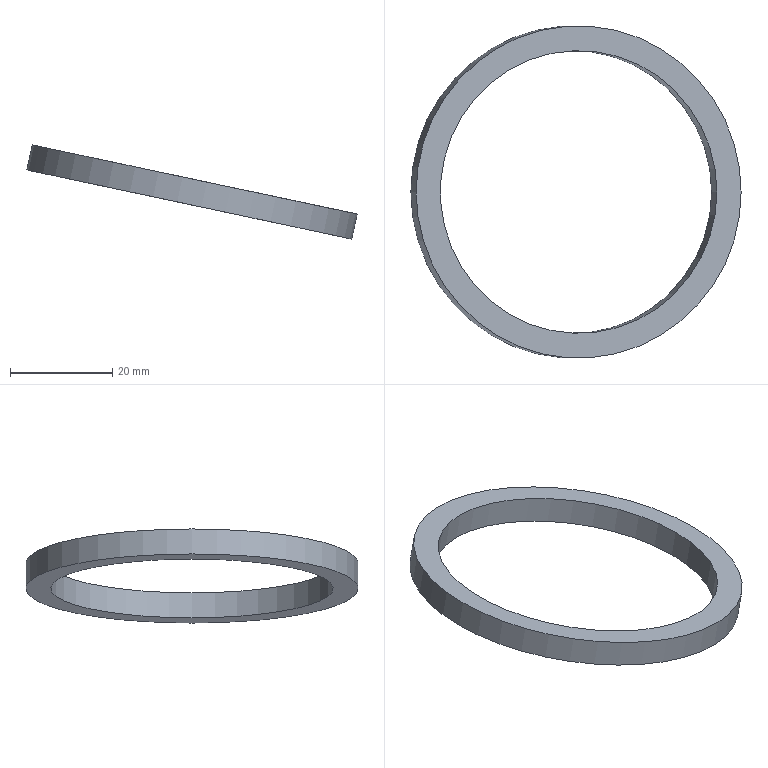Part | STEP file | HL4GZ-1.862.554 (cutter mechanism bushing) | 1 solid | 4 faces | box 64.619 x 65 x 18.405 mm | volume 4582 mm3 | plane 2 | cylinder 2 | commonest cylinder face diameters 55.3 x1 65 x1
STEP:
#1=CARTESIAN_POINT('',(0.,0.,0.));
#2=DIRECTION('',(0.,0.,1.));
#3=DIRECTION('',(1.,0.,0.));
#4=AXIS2_PLACEMENT_3D('',#1,#2,#3);
#5=CARTESIAN_POINT('',(1999.118,0.00003081,-382.69));
#6=VERTEX_POINT('',#5);
#7=CARTESIAN_POINT('',(1972.072,0.00003081,-376.941));
#8=DIRECTION('',(-0.2079,0.,-0.9781));
#9=DIRECTION('',(0.9781,0.,-0.2079));
#10=AXIS2_PLACEMENT_3D('',#7,#8,#9);
#11=CIRCLE('',#10,27.65);
#12=CARTESIAN_POINT('',(1972.072,0.00003081,-376.941));
#13=DIRECTION('',(0.2079,0.,0.9781));
#14=DIRECTION('',(0.,-1.,0.));
#15=AXIS2_PLACEMENT_3D('',#12,#13,#14);
#16=PLANE('',#15);
#17=CARTESIAN_POINT('',(0.,27.65));
#18=CARTESIAN_POINT('',(47.891,27.65));
#19=CARTESIAN_POINT('',(23.946,-13.825));
#20=CARTESIAN_POINT('',(0.,-55.3));
#21=CARTESIAN_POINT('',(-23.946,-13.825));
#22=CARTESIAN_POINT('',(-47.891,27.65));
#23=CARTESIAN_POINT('',(0.,27.65));
#24=(BOUNDED_CURVE()B_SPLINE_CURVE(2,(#17,#18,#19,#20,#21,#22,#23),.UNSPECIFIED.,.T.,.F.)B_SPLINE_CURVE_WITH_KNOTS((1,2,2,2,2,1),(-2.094,0.,2.094,4.189,6.283,8.378),.UNSPECIFIED.)CURVE()GEOMETRIC_REPRESENTATION_ITEM()RATIONAL_B_SPLINE_CURVE((1.,0.5,1.,0.5,1.,0.5,1.))REPRESENTATION_ITEM(''));
#25=(GEOMETRIC_REPRESENTATION_CONTEXT(2)PARAMETRIC_REPRESENTATION_CONTEXT()REPRESENTATION_CONTEXT('',''));
#26=DEFINITIONAL_REPRESENTATION('',(#24),#25);
#27=PCURVE('',#16,#26);
#28=CARTESIAN_POINT('',(1971.033,0.00003081,-381.832));
#29=DIRECTION('',(0.2079,0.,0.9781));
#30=DIRECTION('',(0.,1.,0.));
#31=AXIS2_PLACEMENT_3D('',#28,#29,#30);
#32=CYLINDRICAL_SURFACE('',#31,27.65);
#33=CARTESIAN_POINT('',(10.996,5.));
#34=DIRECTION('',(-1.,0.));
#35=VECTOR('',#34,1.);
#36=LINE('',#33,#35);
#37=(GEOMETRIC_REPRESENTATION_CONTEXT(2)PARAMETRIC_REPRESENTATION_CONTEXT()REPRESENTATION_CONTEXT('',''));
#38=DEFINITIONAL_REPRESENTATION('',(#36),#37);
#39=PCURVE('',#32,#38);
#40=SURFACE_CURVE('',#11,(#27,#39),.PCURVE_S1.);
#41=EDGE_CURVE('',#6,#6,#40,.T.);
#42=ORIENTED_EDGE('',*,*,#41,.T.);
#43=EDGE_LOOP('',(#42));
#44=FACE_BOUND('',#43,.T.);
#45=CARTESIAN_POINT('',(2003.862,0.00003081,-383.698));
#46=VERTEX_POINT('',#45);
#47=CARTESIAN_POINT('',(1972.072,0.00003081,-376.941));
#48=DIRECTION('',(0.2079,0.,0.9781));
#49=DIRECTION('',(0.9781,0.,-0.2079));
#50=AXIS2_PLACEMENT_3D('',#47,#48,#49);
#51=CIRCLE('',#50,32.5);
#52=CARTESIAN_POINT('',(0.,0.));
#53=DIRECTION('',(0.,1.));
#54=AXIS2_PLACEMENT_2D('',#52,#53);
#55=CIRCLE('',#54,32.5);
#56=(GEOMETRIC_REPRESENTATION_CONTEXT(2)PARAMETRIC_REPRESENTATION_CONTEXT()REPRESENTATION_CONTEXT('',''));
#57=DEFINITIONAL_REPRESENTATION('',(#55),#56);
#58=PCURVE('',#16,#57);
#59=CARTESIAN_POINT('',(1971.033,0.00003081,-381.832));
#60=DIRECTION('',(0.2079,0.,0.9781));
#61=DIRECTION('',(0.,1.,0.));
#62=AXIS2_PLACEMENT_3D('',#59,#60,#61);
#63=CYLINDRICAL_SURFACE('',#62,32.5);
#64=CARTESIAN_POINT('',(4.712,5.));
#65=DIRECTION('',(1.,0.));
#66=VECTOR('',#65,1.);
#67=LINE('',#64,#66);
#68=(GEOMETRIC_REPRESENTATION_CONTEXT(2)PARAMETRIC_REPRESENTATION_CONTEXT()REPRESENTATION_CONTEXT('',''));
#69=DEFINITIONAL_REPRESENTATION('',(#67),#68);
#70=PCURVE('',#63,#69);
#71=SURFACE_CURVE('',#51,(#58,#70),.PCURVE_S1.);
#72=EDGE_CURVE('',#46,#46,#71,.T.);
#73=ORIENTED_EDGE('',*,*,#72,.T.);
#74=EDGE_LOOP('',(#73));
#75=FACE_BOUND('',#74,.T.);
#76=ADVANCED_FACE('',(#44,#75),#16,.T.);
#77=CARTESIAN_POINT('',(1998.079,0.00003081,-387.58));
#78=VERTEX_POINT('',#77);
#79=CARTESIAN_POINT('',(1971.033,0.00003081,-381.832));
#80=DIRECTION('',(0.2079,0.,0.9781));
#81=DIRECTION('',(0.9781,0.,-0.2079));
#82=AXIS2_PLACEMENT_3D('',#79,#80,#81);
#83=CIRCLE('',#82,27.65);
#84=CARTESIAN_POINT('',(1971.033,0.00003081,-381.832));
#85=DIRECTION('',(0.2079,0.,0.9781));
#86=DIRECTION('',(0.,-1.,0.));
#87=AXIS2_PLACEMENT_3D('',#84,#85,#86);
#88=PLANE('',#87);
#89=CARTESIAN_POINT('',(0.,0.));
#90=DIRECTION('',(0.,1.));
#91=AXIS2_PLACEMENT_2D('',#89,#90);
#92=CIRCLE('',#91,27.65);
#93=(GEOMETRIC_REPRESENTATION_CONTEXT(2)PARAMETRIC_REPRESENTATION_CONTEXT()REPRESENTATION_CONTEXT('',''));
#94=DEFINITIONAL_REPRESENTATION('',(#92),#93);
#95=PCURVE('',#88,#94);
#96=CARTESIAN_POINT('',(4.712,0.));
#97=DIRECTION('',(1.,0.));
#98=VECTOR('',#97,1.);
#99=LINE('',#96,#98);
#100=(GEOMETRIC_REPRESENTATION_CONTEXT(2)PARAMETRIC_REPRESENTATION_CONTEXT()REPRESENTATION_CONTEXT('',''));
#101=DEFINITIONAL_REPRESENTATION('',(#99),#100);
#102=PCURVE('',#32,#101);
#103=SURFACE_CURVE('',#83,(#95,#102),.PCURVE_S1.);
#104=EDGE_CURVE('',#78,#78,#103,.T.);
#105=ORIENTED_EDGE('',*,*,#104,.T.);
#106=EDGE_LOOP('',(#105));
#107=FACE_BOUND('',#106,.T.);
#108=CARTESIAN_POINT('',(2002.823,0.00003081,-388.589));
#109=VERTEX_POINT('',#108);
#110=CARTESIAN_POINT('',(1971.033,0.00003081,-381.832));
#111=DIRECTION('',(-0.2079,0.,-0.9781));
#112=DIRECTION('',(0.9781,0.,-0.2079));
#113=AXIS2_PLACEMENT_3D('',#110,#111,#112);
#114=CIRCLE('',#113,32.5);
#115=CARTESIAN_POINT('',(0.,32.5));
#116=CARTESIAN_POINT('',(56.292,32.5));
#117=CARTESIAN_POINT('',(28.146,-16.25));
#118=CARTESIAN_POINT('',(0.,-65.));
#119=CARTESIAN_POINT('',(-28.146,-16.25));
#120=CARTESIAN_POINT('',(-56.292,32.5));
#121=CARTESIAN_POINT('',(0.,32.5));
#122=(BOUNDED_CURVE()B_SPLINE_CURVE(2,(#115,#116,#117,#118,#119,#120,#121),.UNSPECIFIED.,.T.,.F.)B_SPLINE_CURVE_WITH_KNOTS((1,2,2,2,2,1),(-2.094,0.,2.094,4.189,6.283,8.378),.UNSPECIFIED.)CURVE()GEOMETRIC_REPRESENTATION_ITEM()RATIONAL_B_SPLINE_CURVE((1.,0.5,1.,0.5,1.,0.5,1.))REPRESENTATION_ITEM(''));
#123=(GEOMETRIC_REPRESENTATION_CONTEXT(2)PARAMETRIC_REPRESENTATION_CONTEXT()REPRESENTATION_CONTEXT('',''));
#124=DEFINITIONAL_REPRESENTATION('',(#122),#123);
#125=PCURVE('',#88,#124);
#126=CARTESIAN_POINT('',(10.996,0.));
#127=DIRECTION('',(-1.,0.));
#128=VECTOR('',#127,1.);
#129=LINE('',#126,#128);
#130=(GEOMETRIC_REPRESENTATION_CONTEXT(2)PARAMETRIC_REPRESENTATION_CONTEXT()REPRESENTATION_CONTEXT('',''));
#131=DEFINITIONAL_REPRESENTATION('',(#129),#130);
#132=PCURVE('',#63,#131);
#133=SURFACE_CURVE('',#114,(#125,#132),.PCURVE_S1.);
#134=EDGE_CURVE('',#109,#109,#133,.T.);
#135=ORIENTED_EDGE('',*,*,#134,.T.);
#136=EDGE_LOOP('',(#135));
#137=FACE_BOUND('',#136,.T.);
#138=ADVANCED_FACE('',(#107,#137),#88,.F.);
#139=ORIENTED_EDGE('',*,*,#134,.F.);
#140=CARTESIAN_POINT('',(2002.823,0.00003081,-388.589));
#141=CARTESIAN_POINT('',(2003.862,0.00003081,-383.698));
#142=B_SPLINE_CURVE_WITH_KNOTS('',1,(#140,#141),.UNSPECIFIED.,.F.,.F.,(2,2),(0.,5.),.PIECEWISE_BEZIER_KNOTS.);
#143=CARTESIAN_POINT('',(10.996,0.));
#144=DIRECTION('',(0.,1.));
#145=VECTOR('',#144,1.);
#146=LINE('',#143,#145);
#147=(GEOMETRIC_REPRESENTATION_CONTEXT(2)PARAMETRIC_REPRESENTATION_CONTEXT()REPRESENTATION_CONTEXT('',''));
#148=DEFINITIONAL_REPRESENTATION('',(#146),#147);
#149=PCURVE('',#63,#148);
#150=CARTESIAN_POINT('',(4.712,0.));
#151=DIRECTION('',(0.,1.));
#152=VECTOR('',#151,1.);
#153=LINE('',#150,#152);
#154=(GEOMETRIC_REPRESENTATION_CONTEXT(2)PARAMETRIC_REPRESENTATION_CONTEXT()REPRESENTATION_CONTEXT('',''));
#155=DEFINITIONAL_REPRESENTATION('',(#153),#154);
#156=PCURVE('',#63,#155);
#157=SEAM_CURVE('',#142,(#149,#156),.PCURVE_S1.);
#158=EDGE_CURVE('',#109,#46,#157,.T.);
#159=ORIENTED_EDGE('',*,*,#158,.T.);
#160=ORIENTED_EDGE('',*,*,#72,.F.);
#161=ORIENTED_EDGE('',*,*,#158,.F.);
#162=EDGE_LOOP('',(#139,#159,#160,#161));
#163=FACE_BOUND('',#162,.T.);
#164=ADVANCED_FACE('',(#163),#63,.T.);
#165=ORIENTED_EDGE('',*,*,#104,.T.);
#166=CARTESIAN_POINT('',(1998.079,0.00003081,-387.58));
#167=CARTESIAN_POINT('',(1999.118,0.00003081,-382.69));
#168=B_SPLINE_CURVE_WITH_KNOTS('',1,(#166,#167),.UNSPECIFIED.,.F.,.F.,(2,2),(0.,5.),.PIECEWISE_BEZIER_KNOTS.);
#169=CARTESIAN_POINT('',(10.996,0.));
#170=DIRECTION('',(0.,1.));
#171=VECTOR('',#170,1.);
#172=LINE('',#169,#171);
#173=(GEOMETRIC_REPRESENTATION_CONTEXT(2)PARAMETRIC_REPRESENTATION_CONTEXT()REPRESENTATION_CONTEXT('',''));
#174=DEFINITIONAL_REPRESENTATION('',(#172),#173);
#175=PCURVE('',#32,#174);
#176=CARTESIAN_POINT('',(4.712,0.));
#177=DIRECTION('',(0.,1.));
#178=VECTOR('',#177,1.);
#179=LINE('',#176,#178);
#180=(GEOMETRIC_REPRESENTATION_CONTEXT(2)PARAMETRIC_REPRESENTATION_CONTEXT()REPRESENTATION_CONTEXT('',''));
#181=DEFINITIONAL_REPRESENTATION('',(#179),#180);
#182=PCURVE('',#32,#181);
#183=SEAM_CURVE('',#168,(#175,#182),.PCURVE_S1.);
#184=EDGE_CURVE('',#78,#6,#183,.T.);
#185=ORIENTED_EDGE('',*,*,#184,.T.);
#186=ORIENTED_EDGE('',*,*,#41,.T.);
#187=ORIENTED_EDGE('',*,*,#184,.F.);
#188=EDGE_LOOP('',(#165,#185,#186,#187));
#189=FACE_BOUND('',#188,.F.);
#190=ADVANCED_FACE('',(#189),#32,.F.);
#191=CLOSED_SHELL('',(#76,#138,#164,#190));
#192=MANIFOLD_SOLID_BREP('',#191);
#193=(LENGTH_UNIT()NAMED_UNIT(*)SI_UNIT(.MILLI.,.METRE.));
#194=UNCERTAINTY_MEASURE_WITH_UNIT(LENGTH_MEASURE(0.00001),#193,'','');
#195=(NAMED_UNIT(*)PLANE_ANGLE_UNIT()SI_UNIT($,.RADIAN.));
#196=(NAMED_UNIT(*)SI_UNIT($,.STERADIAN.)SOLID_ANGLE_UNIT());
#197=(GEOMETRIC_REPRESENTATION_CONTEXT(3)GLOBAL_UNCERTAINTY_ASSIGNED_CONTEXT((#194))GLOBAL_UNIT_ASSIGNED_CONTEXT((#193,#195,#196))REPRESENTATION_CONTEXT('',''));
#198=ADVANCED_BREP_SHAPE_REPRESENTATION('',(#4,#192),#197);